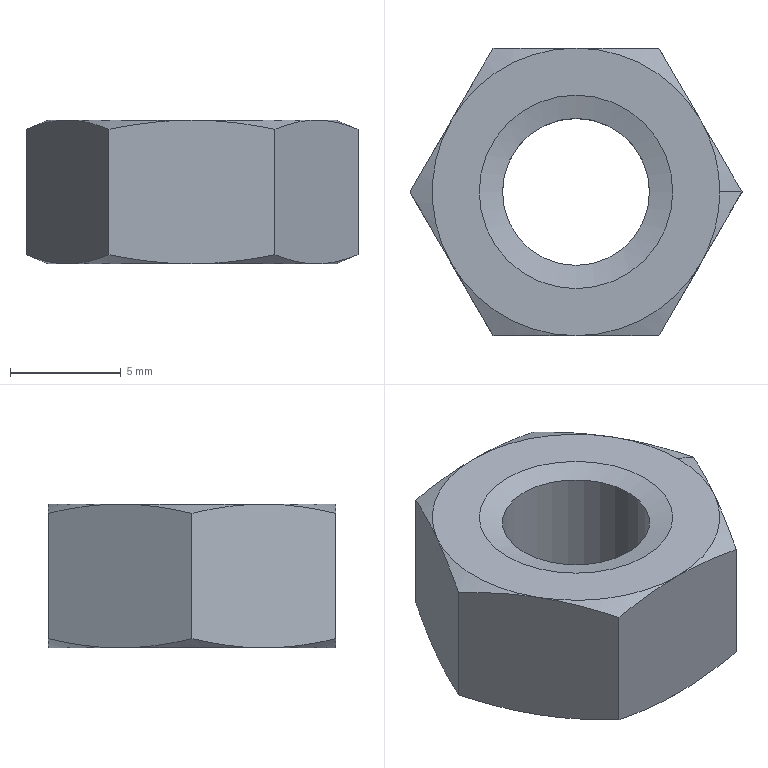Part | STEP file | Left | 1 solid | 25 faces | box 15.011 x 13 x 6.5 mm | volume 715.522 mm3 | cone 16 | plane 8 | cylinder 1 | commonest cylinder face diameters 6.647 x1